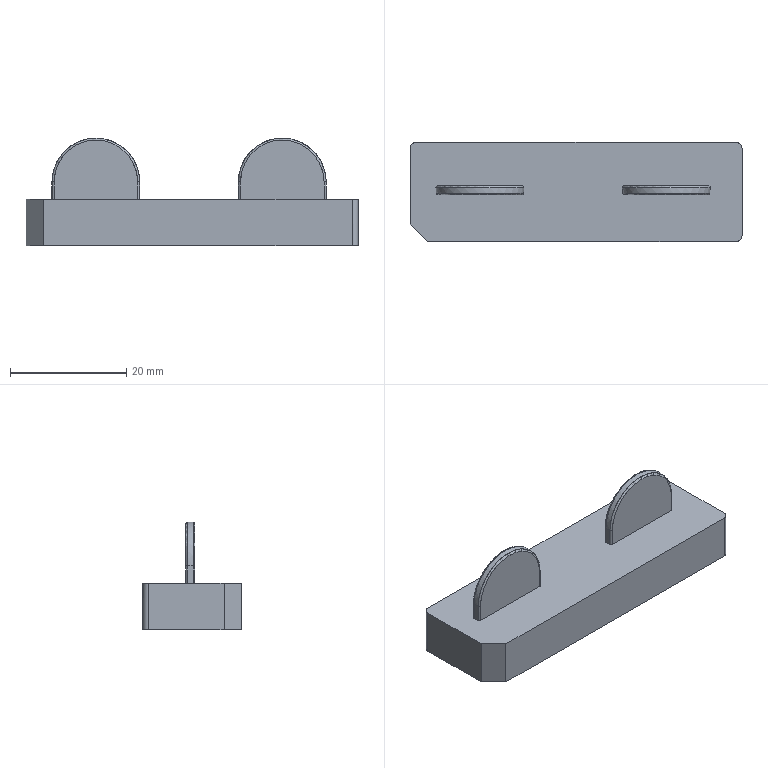NC program | PowerMill | posted by the shop | part box 57 x 17 x 18.538 mm
Lines 1 to 1590 of 218548:
%
G40 G49 G17 G80
( TOOL ID   D10C_1_1_1 )
( TOOL DIA. 10. TIP RAD 0 LENGTH 74. )
( Z = -.073 )
T1 M6
T2
G91 G28 Z0
G0 G90 G54
M08
S8000 M3
G0 X0 Y0 M8
G43 Z10.2 H1
X31.28 Y11.28
Z1.127
G1 Z-.073 F6000
X-31.28 F10000
Y5.64
X31.28
Y0
X-31.28
Y-5.64
X31.28
Y-11.28
X-31.28
X-36.28
G0 Z10.2
X-.267 Y0
Z9.877
X-21.257 Y16.555
Z.691
G1 Z-.509 F6000
Y16.028 F10000
G3 X-16.51 Y11.28 I4.747 J0
G1 X15.17
X15.202 Y6.305
X16.362 Y6.312
X17.135 Y6.289
X17.909 Y6.213
X18.682 Y6.067
X19.455 Y5.831
X20.229 Y5.467
X20.914 Y5.027
X21.748 Y4.254
X22.306 Y3.48
X22.549 Y3.034
X22.698 Y2.707
X22.949 Y1.934
X23.072 Y1.16
X23.082 Y.387
X22.974 Y-.387
X22.8 Y-1.16
X22.593 Y-1.934
X22.251 Y-2.707
X21.776 Y-3.427
X21.002 Y-4.246
X20.229 Y-4.81
X19.833 Y-5.027
X19.455 Y-5.195
X18.682 Y-5.457
X17.909 Y-5.621
X17.135 Y-5.716
X15.588 Y-5.762
X14.041 Y-5.73
X13.268 Y-5.647
X12.495 Y-5.505
X11.721 Y-5.265
X10.948 Y-4.913
X10.174 Y-4.395
X10.006 Y-4.254
X9.265 Y-3.48
X8.747 Y-2.707
X8.404 Y-1.934
X8.198 Y-1.16
X8.023 Y-.387
X7.92 Y.387
X7.926 Y1.16
X8.051 Y1.934
X8.3 Y2.707
X8.627 Y3.362
X9.25 Y4.254
X9.401 Y4.416
X10.086 Y5.027
X10.948 Y5.562
X11.721 Y5.894
X12.495 Y6.108
X13.268 Y6.234
X14.041 Y6.297
X15.202 Y6.305
X15.17 Y11.28
X30.28
G2 X31.28 Y10.28 I0 J-1.
G1 Y-6.113
X26.364
G2 X26.022 Y-6.113 I-.171 J0
X26.364 Y-6.113 I.171 J0
G1 X31.28
Y-10.28
G2 X30.28 Y-11.28 I-1. J0
G1 X-.496
Y-6.67
X-4.031
G2 X-5.467 Y-4.646 I0 J1.521
G1 X-4.986 Y-3.275
G3 X-4.33 Y.083 I-11.234 J3.938
G1 X-4.323 Y.231
G3 X-4.647 Y3.267 I-9.87 J.481
G1 X-5.018 Y4.652
G2 X-3.468 Y6.67 I1.549 J.415
G1 X2.484
G2 X4.023 Y4.665 I0 J-1.593
G1 X3.655 Y3.295
G3 X3.339 Y1.203 I9.192 J-2.463
G1 X3.33 Y.988
G3 X3.998 Y-3.302 I11.284 J-.441
G1 X4.476 Y-4.62
G2 X3.038 Y-6.67 I-1.437 J-.521
G1 X-.496
Y-11.28
X-30.814
G2 X-31.814 Y-10.28 I0 J1.
G1 Y10.28
G2 X-30.814 Y11.28 I1. J0
G1 X-16.51
X-16.509 Y6.309
X-15.349 Y6.31
X-14.575 Y6.264
X-13.802 Y6.167
X-13.029 Y5.989
X-12.255 Y5.712
X-11.482 Y5.293
X-11.086 Y5.027
X-10.708 Y4.716
X-10.25 Y4.254
X-9.935 Y3.85
X-9.692 Y3.48
X-9.301 Y2.707
X-9.161 Y2.33
X-9.051 Y1.934
X-8.926 Y1.16
X-8.918 Y.387
X-9.025 Y-.387
X-9.404 Y-1.934
X-9.747 Y-2.707
X-9.935 Y-3.018
X-10.263 Y-3.48
X-10.708 Y-3.968
X-11.006 Y-4.254
X-11.482 Y-4.625
X-12.167 Y-5.027
X-13.029 Y-5.371
X-13.802 Y-5.573
X-14.575 Y-5.688
X-15.349 Y-5.742
X-16.122 Y-5.759
X-17.669 Y-5.742
X-18.443 Y-5.685
X-19.216 Y-5.569
X-19.989 Y-5.366
X-20.763 Y-5.061
X-21.536 Y-4.612
X-21.994 Y-4.254
X-22.31 Y-3.956
X-22.735 Y-3.48
X-23.083 Y-2.99
X-23.252 Y-2.707
X-23.594 Y-1.934
X-23.802 Y-1.16
X-23.977 Y-.387
X-24.08 Y.387
X-24.074 Y1.16
X-23.949 Y1.934
X-23.857 Y2.273
X-23.699 Y2.707
X-23.305 Y3.48
X-23.083 Y3.822
X-22.747 Y4.254
X-22.31 Y4.7
X-21.914 Y5.027
X-21.536 Y5.282
X-20.763 Y5.704
X-19.989 Y5.984
X-19.216 Y6.164
X-18.443 Y6.262
X-17.669 Y6.309
X-16.509
X-16.51 Y11.28
G0 Z3.305
G1 X-21.257 Y16.555
G0 Z.305
G1 Z-.895 F6000
Y16.028 F10000
G3 X-16.51 Y11.28 I4.747 J0
G1 X12.37
X12.495 Y6.293
X13.268 Y6.312
X17.909
X18.682 Y6.275
X19.455 Y6.15
X20.229 Y5.93
X20.578 Y5.801
X21.002 Y5.608
X21.776 Y5.13
X22.549 Y4.446
X22.726 Y4.254
X23.282 Y3.48
X23.656 Y2.707
X23.891 Y1.934
X24.015 Y1.16
X24.024 Y.387
X23.816 Y-1.16
X23.61 Y-1.934
X23.323 Y-2.604
X22.768 Y-3.48
X22.549 Y-3.747
X22.048 Y-4.254
X21.776 Y-4.477
X20.897 Y-5.027
X20.229 Y-5.331
X19.455 Y-5.561
X18.682 Y-5.709
X17.909 Y-5.765
X13.268 Y-5.771
X12.495 Y-5.726
X11.721 Y-5.604
X10.948 Y-5.394
X10.174 Y-5.064
X9.401 Y-4.607
X8.952 Y-4.254
X8.627 Y-3.941
X8.232 Y-3.48
X7.733 Y-2.707
X7.39 Y-1.934
X7.184 Y-1.16
X6.976 Y.387
X6.984 Y1.107
X1.484 Y1.41
X1.468 Y1.107
G3 X1.577 Y-1.341 I12.301 J-.678
G1 X1.878 Y-3.413
G2 X-.104 Y-5.7 I-1.979 J-.287
G1 X-.903 Y-5.699
G2 X-2.88 Y-3.413 I.003 J2.
G1 X-2.58 Y-1.333
G3 X-2.47 Y1.097 I-12.248 J1.768
G1 X-2.601 Y3.535
G2 X-.619 Y5.642 I1.997 J.107
G1 X-.411 Y5.643
G2 X1.601 Y3.533 I.015 J-2.
G1 X1.484 Y1.41
X6.984 Y1.107
X6.985 Y1.16
X7.081 Y1.794
X7.344 Y2.707
X7.718 Y3.48
X8.274 Y4.254
X8.627 Y4.623
X9.087 Y5.027
X9.401 Y5.258
X10.174 Y5.693
X10.948 Y5.991
X11.721 Y6.184
X12.495 Y6.293
X12.37 Y11.28
X30.28
G2 X31.28 Y10.28 I0 J-1.
G1 Y-10.28
G2 X30.28 Y-11.28 I-1. J0
G1 X-30.814
G2 X-31.814 Y-10.28 I0 J1.
G1 Y10.28
G2 X-30.814 Y11.28 I1. J0
G1 X-19.891
X-19.409 Y6.29
X-19.216 Y6.308
X-17.675 Y6.309
X-17.669
X-15.349 Y6.31
X-15.343 Y6.309
X-13.802 Y6.31
X-13.029 Y6.237
X-12.255 Y6.082
X-11.482 Y5.823
X-10.708 Y5.45
X-10.085 Y5.027
X-9.274 Y4.254
X-8.718 Y3.48
X-8.388 Y2.809
X-8.109 Y1.934
X-7.985 Y1.16
X-7.976 Y.387
X-8.184 Y-1.16
X-8.391 Y-1.934
X-8.733 Y-2.707
X-9.161 Y-3.382
X-9.952 Y-4.254
X-10.708 Y-4.808
X-11.105 Y-5.027
X-11.482 Y-5.212
X-12.255 Y-5.488
X-13.029 Y-5.666
X-13.802 Y-5.749
X-14.575 Y-5.772
X-18.443
X-19.216 Y-5.748
X-19.989 Y-5.662
X-20.763 Y-5.483
X-21.536 Y-5.204
X-22.31 Y-4.797
X-23.048 Y-4.254
X-23.768 Y-3.48
X-24.267 Y-2.707
X-24.61 Y-1.934
X-24.816 Y-1.16
X-25.024 Y.387
X-25.014 Y1.16
X-24.891 Y1.934
X-24.656 Y2.707
X-24.282 Y3.48
X-23.726 Y4.254
X-23.083 Y4.888
X-22.31 Y5.439
X-21.578 Y5.801
X-20.763 Y6.077
X-19.989 Y6.234
X-19.409 Y6.29
X-19.891 Y11.28
X-16.51
G0 Z2.918
G1 X-21.257 Y16.555
G0 Z-.082
G1 Z-1.282 F6000
Y16.028 F10000
G3 X-16.51 Y11.28 I4.747 J0
G1 X-16.509
Y6.311
X-13.029
X-12.255 Y6.247
X-11.482 Y6.087
X-10.667 Y5.801
X-9.935 Y5.42
X-9.369 Y5.027
X-9.161 Y4.85
X-8.575 Y4.254
X-8.388 Y4.025
X-8.02 Y3.48
X-7.647 Y2.707
X-7.407 Y1.934
X-7.282 Y1.16
X-7.273 Y.387
X-7.466 Y-1.16
X-7.669 Y-1.934
X-8.011 Y-2.707
X-8.499 Y-3.48
X-9.161 Y-4.206
X-9.935 Y-4.798
X-10.316 Y-5.027
X-10.708 Y-5.221
X-11.482 Y-5.497
X-12.255 Y-5.679
X-13.029 Y-5.76
X-14.17
X-14.575 Y-5.772
X-18.443
X-18.848 Y-5.759
X-19.989
X-20.763 Y-5.676
X-21.536 Y-5.491
X-22.31 Y-5.212
X-22.685 Y-5.027
X-23.083 Y-4.787
X-23.785 Y-4.254
X-24.501 Y-3.48
X-24.99 Y-2.707
X-25.329 Y-1.934
X-25.535 Y-1.16
X-25.727 Y.387
X-25.717 Y1.16
X-25.593 Y1.934
X-25.403 Y2.569
X-24.979 Y3.48
X-24.63 Y4.001
X-24.425 Y4.254
X-23.857 Y4.836
X-23.631 Y5.027
X-23.083 Y5.409
X-22.333 Y5.801
X-21.536 Y6.082
X-20.763 Y6.244
X-19.989 Y6.311
X-16.509
Y11.28
X11.623
X11.721 Y6.297
X12.495 Y6.312
X18.682
X19.455 Y6.284
X20.229 Y6.154
X21.002 Y5.933
X21.332 Y5.801
X21.776 Y5.583
X22.549 Y5.09
X23.323 Y4.368
X23.98 Y3.48
X24.353 Y2.707
X24.593 Y1.934
X24.718 Y1.16
X24.727 Y.387
X24.534 Y-1.16
X24.329 Y-1.934
X23.988 Y-2.707
X23.501 Y-3.48
X23.323 Y-3.703
X22.785 Y-4.254
X22.549 Y-4.45
X21.686 Y-5.027
X21.002 Y-5.339
X20.229 Y-5.578
X19.455 Y-5.718
X18.682 Y-5.772
X12.495
X11.721 Y-5.735
X10.948 Y-5.62
X10.174 Y-5.402
X9.401 Y-5.071
X8.627 Y-4.584
X8.215 Y-4.254
X7.854 Y-3.9
X7.499 Y-3.48
X7.081 Y-2.834
X6.669 Y-1.934
X6.464 Y-1.16
X6.29 Y.249
X.741 Y.116
G3 X1.024 Y-2.222 I12.23 J.294
G1 X1.299 Y-3.469
G2 X-.375 Y-5.581 I-1.697 J-.374
G1 X-.572 Y-5.583
G2 X-2.294 Y-3.48 I-.023 J1.737
G1 X-2.017 Y-2.191
G3 X-1.913 Y2.452 I-12.049 J2.592
G1 X-2.124 Y3.704
G2 X-.665 Y5.425 I1.455 J.245
G1 X-.328 Y5.424
G2 X1.122 Y3.701 I-.005 J-1.475
G1 X.911 Y2.465
G3 X.741 Y.116 I12.06 J-2.054
G1 X6.29 Y.249
X6.273 Y.387
X6.282 Y1.16
X6.407 Y1.934
X6.647 Y2.707
X7.02 Y3.48
X7.575 Y4.254
X7.854 Y4.556
X8.369 Y5.027
X8.627 Y5.22
X9.401 Y5.674
X10.174 Y5.994
X10.948 Y6.19
X11.721 Y6.297
X11.623 Y11.28
X30.28
G2 X31.28 Y10.28 I0 J-1.
G1 Y-10.28
G2 X30.28 Y-11.28 I-1. J0
G1 X-30.814
G2 X-31.814 Y-10.28 I0 J1.
G1 Y10.28
G2 X-30.814 Y11.28 I1. J0
G1 X-16.51
G0 Z2.532
G1 X-21.257 Y16.555
G0 Z-.468
G1 Z-1.668 F6000
Y16.028 F10000
G3 X-16.51 Y11.28 I4.747 J0
G1 X15.588
Y6.312
X19.455
X20.229 Y6.269
X21.002 Y6.117
X21.776 Y5.868
X22.549 Y5.477
X23.209 Y5.027
X23.992 Y4.254
X24.545 Y3.48
X24.869 Y2.823
X25.15 Y1.934
X25.272 Y1.16
X25.281 Y.387
X25.104 Y-1.16
X24.899 Y-1.934
X24.567 Y-2.707
X24.083 Y-3.48
X23.369 Y-4.254
X22.549 Y-4.876
X22.291 Y-5.027
X21.776 Y-5.275
X21.002 Y-5.543
X20.229 Y-5.703
X19.455 Y-5.77
X18.697
X18.682 Y-5.771
X12.495 Y-5.772
X12.492
X11.721
X10.948 Y-5.724
X10.174 Y-5.59
X9.401 Y-5.344
X8.709 Y-5.027
X7.854 Y-4.442
X7.631 Y-4.254
X7.081 Y-3.687
X6.917 Y-3.48
X6.433 Y-2.707
X6.102 Y-1.934
X5.897 Y-1.16
X5.721 Y.387
X5.724 Y.678
X-.136 Y.845
G3 X.22 Y-2.504 I12.548 J-.356
G1 X.307 Y-2.855
X.437 Y-3.339
X.589 Y-3.816
X.809 Y-4.461
G2 X.102 Y-5.452 I-.708 J-.243
G1 X-1.101
G2 X-1.815 Y-4.453 I0 J.755
G1 X-1.592 Y-3.802
G3 X-.946 Y-.58 I-11.849 J4.055
G1 X-.898 Y.129
X-.889 Y.449
G3 X-1.31 Y3.769 I-11.317 J.251
G1 X-1.503 Y4.453
G2 X-.747 Y5.452 I.756 J.213
G1 X-.252
G2 X.494 Y4.442 I0 J-.781
G1 X.41 Y4.167
G3 X-.136 Y.845 I12.002 J-3.679
G1 X5.724 Y.678
X5.728 Y1.16
X5.851 Y1.934
X6.082 Y2.707
X6.455 Y3.48
X7.007 Y4.254
X7.791 Y5.027
X8.627 Y5.578
X9.067 Y5.801
X9.401 Y5.936
X10.174 Y6.16
X10.948 Y6.288
X11.721 Y6.312
X15.588
Y11.28
X30.28
G2 X31.28 Y10.28 I0 J-1.
G1 Y-10.28
G2 X30.28 Y-11.28 I-1. J0
G1 X-30.814
G2 X-31.814 Y-10.28 I0 J1.
G1 Y10.28
G2 X-30.814 Y11.28 I1. J0
G1 X-20.802
X-20.763 Y6.306
X-19.989 Y6.312
X-13.802
X-13.425 Y6.311
X-13.029
X-13.015 Y6.31
X-12.255 Y6.308
X-11.482 Y6.225
X-10.708 Y6.04
X-10.068 Y5.801
X-9.161 Y5.297
X-8.791 Y5.027
X-8.388 Y4.668
X-8.008 Y4.254
X-7.615 Y3.733
X-7.455 Y3.48
X-7.082 Y2.707
X-6.851 Y1.934
X-6.728 Y1.16
X-6.719 Y.387
X-6.896 Y-1.16
X-7.102 Y-1.934
X-7.433 Y-2.707
X-7.615 Y-3.031
X-7.917 Y-3.48
X-8.388 Y-4.023
X-8.631 Y-4.254
X-9.161 Y-4.682
X-9.709 Y-5.027
X-9.935 Y-5.143
X-10.708 Y-5.453
X-11.482 Y-5.657
X-12.255 Y-5.755
X-13.029 Y-5.772
X-19.989
X-20.763 Y-5.753
X-21.536 Y-5.654
X-22.31 Y-5.447
X-23.083 Y-5.135
X-23.291 Y-5.027
X-23.857 Y-4.668
X-24.369 Y-4.254
X-24.63 Y-4.005
X-25.083 Y-3.48
X-25.403 Y-3.001
X-25.567 Y-2.707
X-25.899 Y-1.934
X-26.103 Y-1.16
X-26.279 Y.387
X-26.27 Y1.16
X-26.177 Y1.794
X-25.918 Y2.707
X-25.545 Y3.48
X-25.403 Y3.705
X-24.992 Y4.254
X-24.63 Y4.651
X-24.209 Y5.027
X-23.857 Y5.285
X-23.083 Y5.73
X-22.31 Y6.034
X-21.536 Y6.222
X-20.763 Y6.306
X-20.802 Y11.28
X-16.51
G0 Z2.146
G1 X-21.257 Y16.555
G0 Z-.854
G1 Z-2.054 F6000
Y16.028 F10000
G3 X-16.51 Y11.28 I4.747 J0
G1 X-.482
Y4.829
X-.436 Y4.81
X-.417 Y4.765
G2 X-.546 Y4.765 I-.064 J0
G1 X-.527 Y4.81
X-.482 Y4.829
Y11.28
X15.588
Y6.312
X19.455
X19.502 Y6.309
X20.229
X21.002 Y6.232
X21.776 Y6.044
X22.431 Y5.801
X23.323 Y5.298
X23.694 Y5.027
X24.096 Y4.668
X24.476 Y4.254
X24.869 Y3.72
X25.019 Y3.48
X25.392 Y2.707
X25.622 Y1.934
X25.74 Y1.16
X25.749 Y.387
X25.584 Y-1.16
X25.379 Y-1.934
X25.054 Y-2.707
X24.869 Y-3.036
X24.57 Y-3.48
X24.096 Y-4.026
X23.859 Y-4.254
X23.323 Y-4.692
X22.792 Y-5.027
X22.549 Y-5.152
X21.776 Y-5.466
X21.002 Y-5.665
X20.229 Y-5.759
X19.455 Y-5.772
X12.495
X12.417
X11.721
X11.687 Y-5.77
X10.948 Y-5.768
X10.174 Y-5.694
X9.401 Y-5.522
X8.627 Y-5.235
X8.207 Y-5.027
X7.854 Y-4.814
X7.141 Y-4.254
X6.43 Y-3.48
X5.946 Y-2.707
X5.621 Y-1.934
X5.416 Y-1.16
X5.252 Y.387
X5.261 Y1.16
X5.377 Y1.934
X5.608 Y2.707
X5.981 Y3.48
X6.524 Y4.254
X7.081 Y4.834
X7.306 Y5.027
X7.854 Y5.412
X8.569 Y5.801
X9.401 Y6.095
X10.174 Y6.26
X10.948 Y6.312
X11.716
X11.721
X15.588
Y11.28
X30.28
G2 X31.28 Y10.28 I0 J-1.
G1 Y-10.28
G2 X30.28 Y-11.28 I-1. J0
G1 X-.494
Y-5.71
G2 X-1.356 Y-4.848 I0 J.862
X.368 Y-4.848 I.862 J0
X-.494 Y-5.71 I-.862 J0
G1 Y-11.28
X-30.814
G2 X-31.814 Y-10.28 I0 J1.
G1 Y10.28
G2 X-30.814 Y11.28 I1. J0
G1 X-21.672
X-21.536 Y6.291
X-20.763 Y6.312
X-19.99
X-19.989
X-19.397
X-12.255
X-11.482 Y6.292
X-10.708 Y6.173
X-9.935 Y5.948
X-9.569 Y5.801
X-9.161 Y5.596
X-8.388 Y5.089
X-7.615 Y4.359
X-6.981 Y3.48
X-6.608 Y2.707
X-6.377 Y1.934
X-6.26 Y1.16
X-6.251 Y.387
X-6.416 Y-1.16
X-6.621 Y-1.934
X-6.946 Y-2.707
X-7.429 Y-3.48
X-7.615 Y-3.711
X-8.142 Y-4.254
X-8.388 Y-4.47
X-9.207 Y-5.027
X-9.935 Y-5.359
X-10.708 Y-5.605
X-11.482 Y-5.732
X-12.255 Y-5.772
X-20.763
X-21.536 Y-5.73
X-22.31 Y-5.6
X-23.083 Y-5.352
X-23.792 Y-5.027
X-24.63 Y-4.455
X-24.859 Y-4.254
X-25.403 Y-3.691
X-25.571 Y-3.48
X-26.054 Y-2.707
X-26.377 Y-1.934
X-26.584 Y-1.16
X-26.748 Y.387
X-26.739 Y1.16
X-26.623 Y1.934
X-26.392 Y2.707
X-26.177 Y3.188
X-26.019 Y3.48
X-25.476 Y4.254
X-24.693 Y5.027
X-23.857 Y5.586
X-23.432 Y5.801
X-23.083 Y5.941
X-22.31 Y6.169
X-21.536 Y6.291
X-21.672 Y11.28
X-16.51
G0 Z1.76
G1 X-21.257 Y16.555
G0 Z-1.24
G1 Z-2.44 F6000
Y16.028 F10000
G3 X-16.51 Y11.28 I4.747 J0
G1 X-.511
Y5.128
X-.479 Y5.115
X-.466 Y5.083
G2 X-.555 Y5.083 I-.044 J0
G1 X-.542 Y5.115
X-.511 Y5.128
Y11.28
X15.588
Y6.312
X20.229
X21.002 Y6.289
X21.776 Y6.161
X22.549 Y5.926
X22.854 Y5.801
X23.323 Y5.562
X24.096 Y5.038
X24.869 Y4.279
X25.428 Y3.48
X25.643 Y3.07
X25.8 Y2.707
X26.03 Y1.934
X26.151 Y1.16
X26.159 Y.387
X25.999 Y-1.16
X25.795 Y-1.934
X25.643 Y-2.337
X25.471 Y-2.707
X24.989 Y-3.48
X24.281 Y-4.254
X24.096 Y-4.417
X23.214 Y-5.027
X22.549 Y-5.34
X21.776 Y-5.594
X21.002 Y-5.728
X20.229 Y-5.772
X10.948
X10.174 Y-5.747
X9.401 Y-5.634
X8.627 Y-5.409
X7.854 Y-5.063
X7.081 Y-4.562
X6.719 Y-4.254
X6.307 Y-3.84
X6.011 Y-3.48
X5.534 Y-2.717
X5.205 Y-1.934
X5. Y-1.16
X4.841 Y.387
X4.85 Y1.16
X4.97 Y1.934
X5.2 Y2.707
X5.534 Y3.411
X6.109 Y4.254
X6.307 Y4.482
X6.89 Y5.027
X7.081 Y5.172
X7.854 Y5.659
X8.146 Y5.801
X8.627 Y5.989
X9.401 Y6.2
X10.174 Y6.302
X10.948 Y6.312
X15.588
Y11.28
X30.28
G2 X31.28 Y10.28 I0 J-1.
G1 Y-10.28
G2 X30.28 Y-11.28 I-1. J0
G1 X-30.814
G2 X-31.814 Y-10.28 I0 J1.
G1 Y.441
X-27.159 Y.387
X-27.15 Y1.16
X-27.03 Y1.934
X-26.8 Y2.707
X-26.428 Y3.48
X-26.177 Y3.87
X-25.891 Y4.254
X-25.403 Y4.773
X-25.109 Y5.027
X-24.63 Y5.373
X-23.857 Y5.799
X-23.083 Y6.078
X-22.31 Y6.253
X-21.536 Y6.312
X-11.482
X-10.708 Y6.255
X-9.935 Y6.083
X-9.161 Y5.807
X-8.388 Y5.384
X-7.891 Y5.027
X-7.615 Y4.789
X-7.109 Y4.254
X-6.841 Y3.896
X-6.572 Y3.48
X-6.2 Y2.707
X-6.068 Y2.316
X-5.97 Y1.934
X-5.849 Y1.16
X-5.841 Y.387
X-6.001 Y-1.16
X-6.205 Y-1.934
X-6.529 Y-2.707
X-6.707 Y-3.011
X-.991 Y-4.679
G2 X-.254 Y-4.784 I.361 J-.105
X-1.006 Y-4.784 I-.376 J0
G1 X-1.003 Y-4.731
X-.991 Y-4.679
X-6.707 Y-3.011
X-6.841 Y-3.24
X-7.012 Y-3.48
X-7.615 Y-4.155
X-8.388 Y-4.785
X-8.786 Y-5.027
X-9.161 Y-5.214
X-9.935 Y-5.514
X-10.708 Y-5.69
X-11.482 Y-5.767
X-12.255 Y-5.772
X-20.763
X-21.536 Y-5.767
X-22.31 Y-5.687
X-23.083 Y-5.508
X-23.857 Y-5.206
X-24.214 Y-5.027
X-24.63 Y-4.772
X-25.281 Y-4.254
X-25.988 Y-3.48
X-26.177 Y-3.213
X-26.472 Y-2.707
X-26.795 Y-1.934
X-27. Y-1.16
X-27.159 Y.387
X-31.814 Y.441
Y10.28
G2 X-30.814 Y11.28 I1. J0
G1 X-16.51
G0 Z1.374
G1 X-21.257 Y16.555
G0 Z-1.626
G1 Z-2.826 F6000
Y16.028 F10000
G3 X-16.51 Y11.28 I4.747 J0
G1 X-.495
Y5.537
G2 X-.34 Y5.382 I0 J-.155
X-.651 Y5.382 I-.155 J0
X-.495 Y5.537 I.155 J0
G1 Y11.28
X30.28
G2 X31.28 Y10.28 I0 J-1.
G1 Y1.214
X26.501 Y1.16
X26.509 Y.387
X26.437 Y-.387
X26.353 Y-1.16
X26.148 Y-1.934
X25.826 Y-2.707
X25.643 Y-3.036
X25.342 Y-3.48
X24.869 Y-4.026
X24.641 Y-4.254
X24.096 Y-4.699
X23.576 Y-5.027
X23.323 Y-5.158
X22.549 Y-5.479
X21.776 Y-5.672
X21.002 Y-5.763
X20.229 Y-5.772
X19.732
X10.948
X10.918 Y-5.771
X10.174
X9.401 Y-5.7
X8.627 Y-5.534
X7.854 Y-5.24
X7.424 Y-5.027
X7.081 Y-4.819
X6.359 Y-4.254
X5.657 Y-3.48
X5.174 Y-2.707
X4.852 Y-1.934
X4.647 Y-1.16
X4.491 Y.387
X4.501 Y1.16
X4.616 Y1.934
X4.847 Y2.707
X5.218 Y3.48
X5.534 Y3.963
X5.755 Y4.254
X6.307 Y4.832
X6.536 Y5.027
X7.081 Y5.416
X7.786 Y5.801
X8.627 Y6.104
X9.401 Y6.265
X10.174 Y6.312
X10.942
X10.948
X20.229
X20.272 Y6.311
X21.002 Y6.31
X21.776 Y6.238
X22.549 Y6.05
X23.214 Y5.801
X24.096 Y5.297
X24.464 Y5.027
X24.869 Y4.665
X25.245 Y4.254
X25.782 Y3.48
X26.153 Y2.707
X26.384 Y1.934
X26.501 Y1.16
X31.28 Y1.214
Y-10.28
G2 X30.28 Y-11.28 I-1. J0
G1 X-30.814
G2 X-31.814 Y-10.28 I0 J1.
G1 Y.439
X-27.509 Y.387
X-27.5 Y1.16
X-27.383 Y1.934
X-27.153 Y2.707
X-26.95 Y3.169
X-26.782 Y3.48
X-26.245 Y4.254
X-25.464 Y5.027
X-24.63 Y5.591
X-24.214 Y5.801
X-23.857 Y5.946
X-23.083 Y6.178
X-22.31 Y6.295
X-21.536 Y6.312
X-11.482
X-10.708 Y6.297
X-9.935 Y6.182
X-9.161 Y5.952
X-8.786 Y5.801
X-8.388 Y5.6
X-7.615 Y5.087
X-6.841 Y4.356
X-6.218 Y3.48
X-6.068 Y3.204
X-5.846 Y2.707
X-5.616 Y1.934
X-5.499 Y1.16
X-5.491 Y.387
X-5.647 Y-1.16
X-5.852 Y-1.934
X-6.174 Y-2.707
X-6.53 Y-3.277
X-1.149 Y-4.847
G2 X-.178 Y-4.986 I.476 J-.139
X-1.169 Y-4.986 I-.496 J0
G1 X-1.164 Y-4.915
X-1.149 Y-4.847
X-6.53 Y-3.277
X-6.657 Y-3.48
X-6.841 Y-3.711
X-7.36 Y-4.254
X-7.615 Y-4.477
X-8.424 Y-5.027
X-9.161 Y-5.374
X-9.935 Y-5.614
X-10.708 Y-5.742
X-11.482 Y-5.772
X-21.536
X-22.31 Y-5.74
X-23.083 Y-5.61
X-23.857 Y-5.367
X-24.576 Y-5.027
X-25.403 Y-4.463
X-25.641 Y-4.254
X-26.177 Y-3.688
X-26.343 Y-3.48
X-26.824 Y-2.707
X-27.147 Y-1.934
X-27.353 Y-1.16
X-27.509 Y.387
X-31.814 Y.439
Y10.28
G2 X-30.814 Y11.28 I1. J0
G1 X-16.51
G0 Z.988
G1 X-21.257 Y16.555
G0 Z-2.012
G1 Z-3.212 F6000
Y16.028 F10000
G3 X-16.51 Y11.28 I4.747 J0
G1 X-.5
Y6.78
Y11.28
X30.28
G2 X31.28 Y10.28 I0 J-1.
G1 Y1.208
X26.804 Y1.16
X26.812 Y.387
X26.66 Y-1.16
X26.456 Y-1.934
X26.134 Y-2.707
X25.651 Y-3.48
X24.956 Y-4.254
X24.096 Y-4.909
X23.893 Y-5.027
X23.323 Y-5.309
X22.549 Y-5.577
X21.776 Y-5.723
X21.002 Y-5.772
X10.174
X9.401 Y-5.745
X8.627 Y-5.619
X7.854 Y-5.382
X7.107 Y-5.027
X6.307 Y-4.484
X6.044 Y-4.254
X5.534 Y-3.712
X5.349 Y-3.48
X4.866 Y-2.707
X4.543 Y-1.934
X4.339 Y-1.16
X4.187 Y.387
X4.196 Y1.16
X4.317 Y1.934
X4.547 Y2.707
X4.76 Y3.189
X4.918 Y3.48
X5.449 Y4.254
X6.23 Y5.027
X7.081 Y5.605
X7.47 Y5.801
X7.854 Y5.956
X8.627 Y6.186
X9.401 Y6.299
X10.174 Y6.312
X21.002
X21.776 Y6.283
X22.549 Y6.144
X23.323 Y5.888
X24.096 Y5.503
X24.77 Y5.027
X25.551 Y4.254
X26.082 Y3.48
X26.416 Y2.799
X26.684 Y1.934
X26.804 Y1.16
X31.28 Y1.208
Y-10.28
G2 X30.28 Y-11.28 I-1. J0
G1 X-.5
Y-6.78
Y-11.28
X-30.814
G2 X-31.814 Y-10.28 I0 J1.
G1 Y.432
X-27.813 Y.387
X-27.804 Y1.16
X-27.684 Y1.934
X-27.454 Y2.707
X-27.082 Y3.48
X-26.551 Y4.254
X-26.177 Y4.664
X-25.77 Y5.027
X-25.403 Y5.302
X-24.63 Y5.754
X-23.857 Y6.055
X-23.083 Y6.241
X-22.31 Y6.311
X-21.568
X-21.536 Y6.312
X-11.482
X-11.414 Y6.311
X-10.708 Y6.31
X-9.935 Y6.244
X-9.161 Y6.061
X-8.47 Y5.801
X-7.615 Y5.315
X-7.23 Y5.027
X-6.841 Y4.681
X-6.449 Y4.254
X-5.918 Y3.48
X-5.546 Y2.707
X-5.316 Y1.934
X-5.197 Y1.16
X-5.188 Y.387
X-5.294 Y-.868
X-5.34 Y-1.16
X-5.544 Y-1.934
X-5.866 Y-2.707
X-6.068 Y-3.065
X-6.349 Y-3.48
X-6.841 Y-4.053
X-7.044 Y-4.254
X-7.615 Y-4.719
X-8.107 Y-5.027
X-8.388 Y-5.173
X-9.161 Y-5.492
X-9.935 Y-5.679
X-10.708 Y-5.765
X-11.482 Y-5.772
X-21.536
X-22.31 Y-5.765
X-23.083 Y-5.677
X-23.857 Y-5.485
X-24.63 Y-5.164
X-24.893 Y-5.027
X-25.403 Y-4.706
X-25.956 Y-4.254
X-26.177 Y-4.033
X-26.651 Y-3.48
X-26.95 Y-3.036
X-27.133 Y-2.707
X-27.458 Y-1.934
X-27.662 Y-1.16
X-27.724 Y-.705
X-27.813 Y.387
X-31.814 Y.432
Y10.28
G2 X-30.814 Y11.28 I1. J0
G1 X-16.51
G0 Z.601
G1 X-21.257 Y16.555
G0 Z-2.399
G1 Z-3.599 F6000
Y16.028 F10000
G3 X-16.51 Y11.28 I4.747 J0
G1 X-.5
Y6.78
Y11.28
X30.28
G2 X31.28 Y10.28 I0 J-1.
G1 Y1.207
X27.066 Y1.16
X27.075 Y.387
X26.927 Y-1.16
X26.727 Y-1.934
X26.407 Y-2.707
X25.925 Y-3.48
X25.643 Y-3.827
X25.236 Y-4.254
X24.869 Y-4.567
X24.174 Y-5.027
X23.323 Y-5.425
X22.549 Y-5.644
X21.776 Y-5.755
X21.002 Y-5.772
X10.174
X9.401 Y-5.765
X8.627 Y-5.677
X7.854 Y-5.486
X7.081 Y-5.163
X6.307 Y-4.7
X5.764 Y-4.254
X5.534 Y-4.023
X5.075 Y-3.48
X4.76 Y-3.009
X4.593 Y-2.707
X4.274 Y-1.934
X4.073 Y-1.16
X3.926 Y.387
X3.934 Y1.16
X4.048 Y1.934
X4.278 Y2.707
X4.65 Y3.48
X5.177 Y4.254
X5.534 Y4.647
X5.957 Y5.027
X6.307 Y5.294
X7.081 Y5.749
X7.854 Y6.054
X8.627 Y6.24
X9.401 Y6.311
X10.127
X10.174 Y6.312
X20.306
X21.002
X21.776 Y6.305
X22.549 Y6.208
X23.323 Y5.994
X23.81 Y5.801
X24.096 Y5.661
X24.869 Y5.164
X25.043 Y5.027
X25.643 Y4.462
X25.823 Y4.254
X26.35 Y3.48
X26.722 Y2.707
X26.952 Y1.934
X27.066 Y1.16
X31.28 Y1.207
Y-10.28
G2 X30.28 Y-11.28 I-1. J0
G1 X-.5
Y-6.78
Y-11.28
X-30.814
G2 X-31.814 Y-10.28 I0 J1.
G1 Y.428
X-28.075 Y.387
X-28.066 Y1.16
X-27.952 Y1.934
X-27.722 Y2.707
X-27.35 Y3.48
X-26.823 Y4.254
X-26.177 Y4.915
X-25.403 Y5.486
X-24.81 Y5.801
X-23.857 Y6.138
X-23.083 Y6.281
X-22.31 Y6.312
X-10.708
X-9.935 Y6.283
X-9.161 Y6.142
X-8.388 Y5.884
X-7.615 Y5.497
X-6.957 Y5.027
X-6.177 Y4.254
X-5.65 Y3.48
X-5.294 Y2.747
X-5.048 Y1.934
X-4.934 Y1.16
X-4.925 Y.387
X-5.073 Y-1.16
X-5.273 Y-1.934
X-5.593 Y-2.707
X-6.068 Y-3.47
X-6.764 Y-4.254
X-7.615 Y-4.903
X-7.826 Y-5.027
X-8.388 Y-5.309
X-9.161 Y-5.577
X-9.935 Y-5.724
X-10.708 Y-5.772
X-22.31
X-23.083 Y-5.722
X-23.857 Y-5.572
X-24.63 Y-5.301
X-25.403 Y-4.892
X-26.177 Y-4.307
X-26.925 Y-3.48
X-27.407 Y-2.707
X-27.727 Y-1.934
X-27.927 Y-1.16
X-28.075 Y.387
X-31.814 Y.428
Y10.28
G2 X-30.814 Y11.28 I1. J0
G1 X-16.51
G0 Z.215
G1 X-21.257 Y16.555
G0 Z-2.785
G1 Z-3.985 F6000
Y16.028 F10000
G3 X-16.51 Y11.28 I4.747 J0
G1 X-.501
Y6.78
Y11.28
X30.28
G2 X31.28 Y10.28 I0 J-1.
G1 Y1.205
X27.308 Y1.16
X27.317 Y.387
X27.19 Y-1.054
X26.97 Y-1.934
X26.651 Y-2.707
X26.416 Y-3.122
X26.171 Y-3.48
X25.643 Y-4.096
X25.481 Y-4.254
X24.869 Y-4.748
X24.419 Y-5.027
X24.096 Y-5.198
X23.323 Y-5.508
X22.549 Y-5.688
X21.776 Y-5.769
X21.002 Y-5.772
X9.401
X8.627 Y-5.715
X7.854 Y-5.559
X7.081 Y-5.281
X6.307 Y-4.864
X5.534 Y-4.268
X4.83 Y-3.48
X4.348 Y-2.707
X4.029 Y-1.934
X3.829 Y-1.16
X3.684 Y.387
X3.692 Y1.16
X3.807 Y1.934
X3.987 Y2.567
X4.408 Y3.48
X4.76 Y4.029
X4.934 Y4.254
X5.534 Y4.876
X6.307 Y5.459
X6.944 Y5.801
X7.854 Y6.126
X8.627 Y6.276
X9.401 Y6.312
X21.776
X22.549 Y6.251
X23.323 Y6.076
X24.056 Y5.801
X24.869 Y5.343
X25.287 Y5.027
X25.643 Y4.714
X26.067 Y4.254
X26.416 Y3.774
X26.592 Y3.48
X26.962 Y2.707
X27.19 Y1.945
X27.308 Y1.16
X31.28 Y1.205
Y-10.28
G2 X30.28 Y-11.28 I-1. J0
G1 X-.501
Y-6.78
Y-11.28
X-30.814
G2 X-31.814 Y-10.28 I0 J1.
G1 Y-.135
X-28.298 Y.193
X-28.316 Y.387
X-28.308 Y1.16
X-28.192 Y1.934
X-27.962 Y2.707
X-27.592 Y3.48
X-27.066 Y4.254
X-26.95 Y4.391
X-26.287 Y5.027
X-25.403 Y5.628
X-25.056 Y5.801
X-24.63 Y5.97
X-23.857 Y6.197
X-23.083 Y6.3
X-22.31 Y6.312
X-10.708
X-9.935 Y6.301
X-9.161 Y6.2
X-8.388 Y5.977
X-7.944 Y5.801
X-7.615 Y5.638
X-6.841 Y5.131
X-6.068 Y4.412
X-5.933 Y4.254
X-5.408 Y3.48
X-5.038 Y2.707
X-4.808 Y1.934
X-4.692 Y1.16
X-4.683 Y.387
X-4.829 Y-1.16
X-5.03 Y-1.934
X-5.294 Y-2.599
X-5.831 Y-3.48
X-6.068 Y-3.775
X-6.519 Y-4.254
X-6.841 Y-4.533
X-7.58 Y-5.027
X-8.388 Y-5.408
X-9.161 Y-5.634
X-9.935 Y-5.752
X-10.708 Y-5.772
X-22.31
X-23.083 Y-5.75
X-23.857 Y-5.631
X-24.63 Y-5.401
X-25.42 Y-5.027
X-26.177 Y-4.519
X-26.482 Y-4.254
X-26.95 Y-3.755
X-27.17 Y-3.48
X-27.652 Y-2.707
X-27.971 Y-1.934
X-28.171 Y-1.16
X-28.298 Y.193
X-31.814 Y-.135
Y10.28
G2 X-30.814 Y11.28 I1. J0
G1 X-16.51
G0 Z-.171
G1 X-21.257 Y16.555
G0 Z-3.171
G1 Z-4.371 F6000
Y16.028 F10000
G3 X-16.51 Y11.28 I4.747 J0
G1 X-.495
Y6.78
Y11.28
X30.28
G2 X31.28 Y10.28 I0 J-1.
G1 Y1.202
X27.509 Y1.16
X27.517 Y.387
X27.374 Y-1.16
X27.19 Y-1.883
X26.854 Y-2.707
X26.416 Y-3.42
X25.687 Y-4.254
X24.869 Y-4.883
X24.626 Y-5.027
X24.096 Y-5.297
X23.323 Y-5.57
X22.549 Y-5.723
X21.776 Y-5.772
X9.401
X8.627 Y-5.744
X7.854 Y-5.614
X7.081 Y-5.371
X6.374 Y-5.027
X5.534 Y-4.449
X5.313 Y-4.254
X4.628 Y-3.48
X4.146 Y-2.707
X3.987 Y-2.363
X3.827 Y-1.934
X3.627 Y-1.16
X3.483 Y.387
X3.491 Y1.16
X3.606 Y1.934
X3.837 Y2.707
X3.987 Y3.059
X4.207 Y3.48
X4.732 Y4.254
X5.51 Y5.027
X6.307 Y5.582
X6.739 Y5.801
X7.081 Y5.943
X7.854 Y6.181
X8.627 Y6.296
X9.401 Y6.312
X21.776
X22.549 Y6.28
X23.323 Y6.137
X24.096 Y5.871
X24.869 Y5.477
X25.643 Y4.898
X26.268 Y4.254
X26.416 Y4.064
X26.793 Y3.48
X27.163 Y2.707
X27.394 Y1.934
X27.509 Y1.16
X31.28 Y1.202
Y-10.28
G2 X30.28 Y-11.28 I-1. J0
G1 X-.5
Y-6.78
Y-11.28
X-30.814
G2 X-31.814 Y-10.28 I0 J1.
G1 Y.423
X-28.517 Y.387
X-28.508 Y1.16
X-28.394 Y1.934
X-28.163 Y2.707
X-27.793 Y3.48
X-27.268 Y4.254
X-26.95 Y4.608
X-26.49 Y5.027
X-26.177 Y5.271
X-25.403 Y5.733
X-24.63 Y6.048
X-23.857 Y6.237
X-23.083 Y6.31
X-22.445
X-22.31 Y6.312
X-10.708
X-10.656 Y6.311
X-9.935
X-9.161 Y6.241
X-8.388 Y6.053
X-7.739 Y5.801
X-6.841 Y5.284
X-6.51 Y5.027
X-6.068 Y4.627
X-5.733 Y4.254
X-5.294 Y3.631
X-4.837 Y2.707
X-4.607 Y1.934
X-4.492 Y1.16
X-4.483 Y.387
X-4.626 Y-1.16
X-4.827 Y-1.934
X-5.146 Y-2.707
X-5.294 Y-2.976
X-5.628 Y-3.48
X-6.068 Y-4.007
X-6.313 Y-4.254
X-6.841 Y-4.688
X-7.374 Y-5.027
X-7.615 Y-5.157
X-8.388 Y-5.483
X-9.161 Y-5.676
X-9.935 Y-5.765
X-10.708 Y-5.772
X-22.31
X-23.083 Y-5.764
X-23.857 Y-5.673
X-24.63 Y-5.477
X-25.403 Y-5.15
X-26.177 Y-4.675
X-26.687 Y-4.254
X-26.95 Y-3.987
X-27.372 Y-3.48